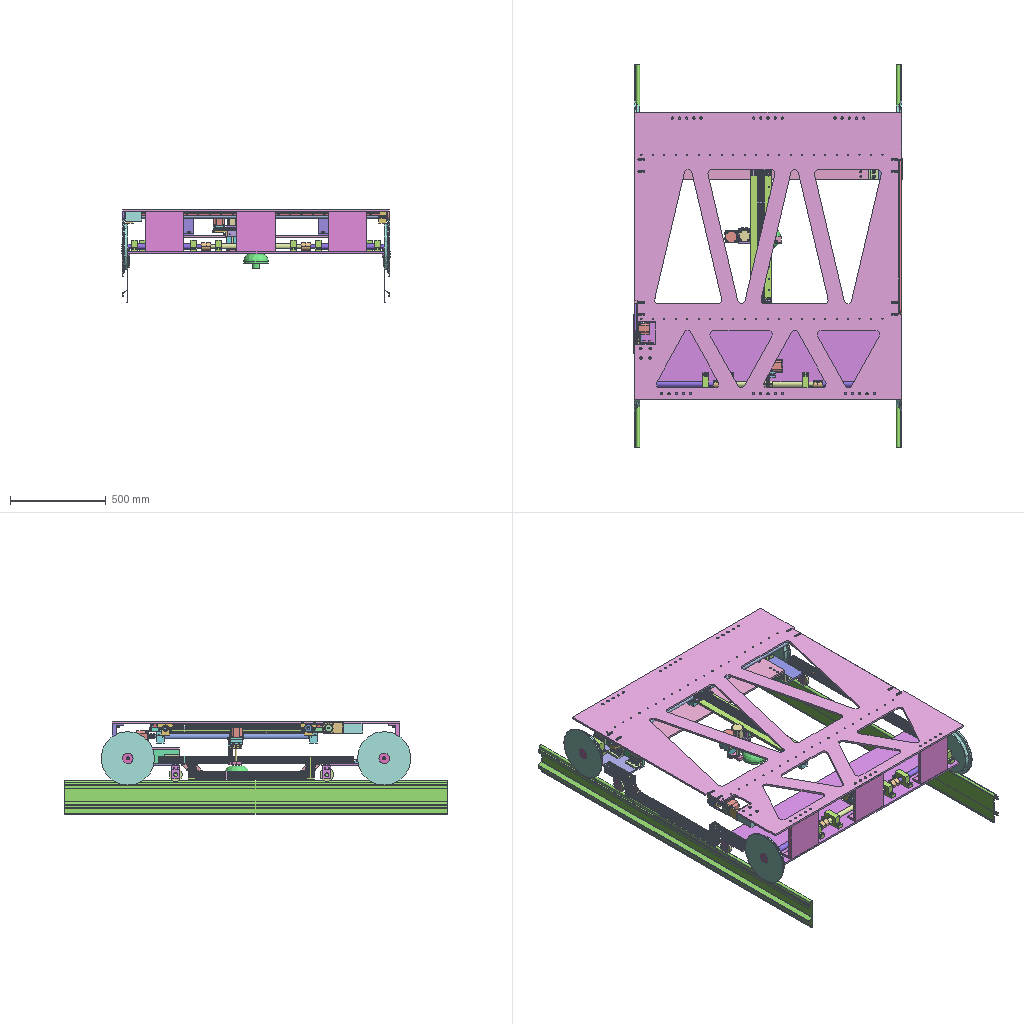Assembly | NX | 100 different items | 711 placed | box 1401 x 2000 x 485 mm
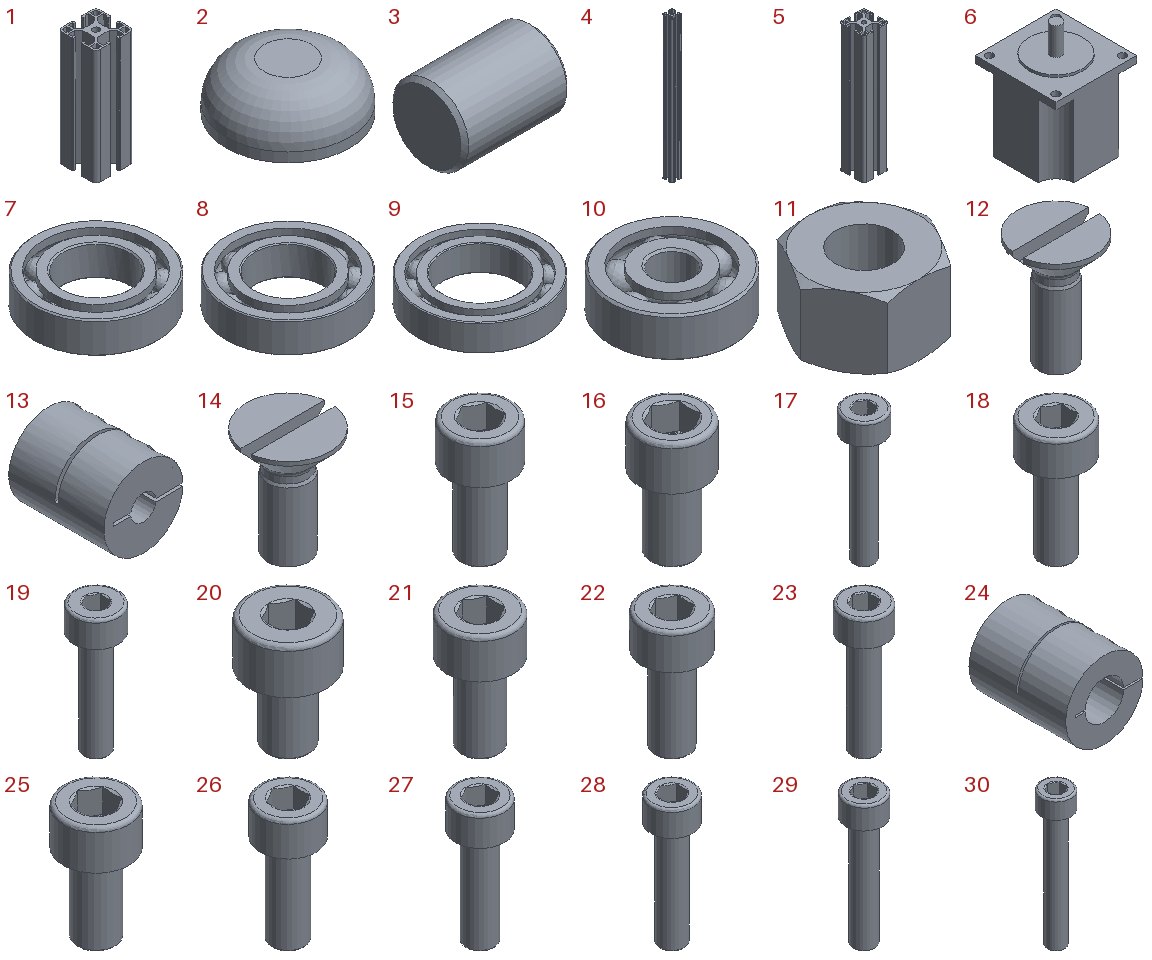Parts list (item | quantity | size | volume | features):
1 | x2 | 40 x 40 x 120 mm | 69185 mm3 | features DATUM_CSYS 2, EXTRUDE 1, SKETCH 1
2 | x1 | 130 x 130 x 80 mm | 580405 mm3 | features DATUM_CSYS 2, SKETCH 1, SWP104 1
3 | x4 | 28 x 20 x 20 mm | 8736 mm3 | features DATUM_CSYS 2, CHAMFER 1, EXTRUDE 1, SKETCH 1
4 | x1 | 40 x 40 x 580 mm | 334396 mm3 | features DATUM_CSYS 2, EXTRUDE 1, SKETCH 1
5 | x1 | 40 x 40 x 205 mm | 118192 mm3 | features DATUM_CSYS 2, EXTRUDE 1, SKETCH 1
6 | x4 | 57 x 57 x 76.9 mm | 158968 mm3 | features 57BYG350CL-SASSML-0601步进电机.SLDPRT 2
7 | x1 | 28 x 28 x 7 mm | 2050 mm3 | features SWP104 15, INSTANCE_SET 9, CHAMFER 3, SKETCH 3, DATUM_CSYS 2, FSET 2, CIRCULAR_PATTERN 1, LINE 1
8 | x6 | 37 x 37 x 9 mm | 4662 mm3 | features SWP104 16, INSTANCE_SET 10, CHAMFER 3, SKETCH 3, DATUM_CSYS 2, FSET 2, CIRCULAR_PATTERN 1, LINE 1
9 | x10 | 42 x 42 x 9 mm | 5487 mm3 | features SWP104 18, INSTANCE_SET 12, CHAMFER 3, SKETCH 3, DATUM_CSYS 2, FSET 2, CIRCULAR_PATTERN 1, LINE 1
10 | x1 | 19 x 19 x 6 mm | 1034 mm3 | features SWP104 11, INSTANCE_SET 5, CHAMFER 3, SKETCH 3, DATUM_CSYS 2, FSET 2, CIRCULAR_PATTERN 1, LINE 1
11 | x84 | 11.547 x 10 x 6.4 mm | 416.752 mm3 | features META 3, SKETCH 3, DATUM_CSYS 2, EXTRUDE 2, SWP104 2, LINE 1, SYMBOLIC_THREAD 1, THREADS 1
12 | x1 | 8.314 x 8.4 x 12 mm | 190.86 mm3 | features DATUM_CSYS 2, SKETCH 2, EXTRUDE 1, LINE 1, META 1, SWP104 1, SYMBOLIC_THREAD 1, THREADS 1
13 | x1 | 24.99 x 30 x 25 mm | 10501 mm3 | features SIMPLE HOLE 14, DATUM_CSYS 6, SYMBOLIC_THREAD 6, SKETCH 5, EXTRUDE 4, HOLE PACKAGE 3, ASSOCIATIVE_INTERSECTION 1, SWP104 1
14 | x4 | 15.673 x 15.8 x 20 mm | 1245 mm3 | features DATUM_CSYS 2, SKETCH 2, EXTRUDE 1, LINE 1, META 1, SWP104 1, SYMBOLIC_THREAD 1, THREADS 1
15 | x77 | 16 x 16 x 30 mm | 3113 mm3 | features SKETCH 3, BLEND 2, DATUM_CSYS 2, META 2, SWP104 2, CHAMFER 1, EXTRUDE 1, LINE 1, SYMBOLIC_THREAD 1, THREADS 1
16 | x55 | 18 x 18 x 32 mm | 4482 mm3 | features SKETCH 3, BLEND 2, DATUM_CSYS 2, META 2, SWP104 2, CHAMFER 1, EXTRUDE 1, LINE 1, SYMBOLIC_THREAD 1, THREADS 1
17 | x4 | 5.5 x 5.5 x 19 mm | 163.401 mm3 | features SKETCH 3, BLEND 2, DATUM_CSYS 2, META 2, SWP104 2, CHAMFER 1, EXTRUDE 1, LINE 1, SYMBOLIC_THREAD 1, THREADS 1
18 | x3 | 5.5 x 5.5 x 11 mm | 111.507 mm3 | features SKETCH 3, BLEND 2, DATUM_CSYS 2, META 2, SWP104 2, CHAMFER 1, EXTRUDE 1, LINE 1, SYMBOLIC_THREAD 1, THREADS 1
19 | x2 | 7 x 7 x 20 mm | 315.757 mm3 | features SKETCH 3, BLEND 2, DATUM_CSYS 2, META 2, SWP104 2, CHAMFER 1, EXTRUDE 1, LINE 1, SYMBOLIC_THREAD 1, THREADS 1
20 | x4 | 7 x 7 x 10 mm | 200.071 mm3 | features SKETCH 3, BLEND 2, DATUM_CSYS 2, META 2, SWP104 2, CHAMFER 1, EXTRUDE 1, LINE 1, SYMBOLIC_THREAD 1, THREADS 1
21 | x30 | 8.5 x 8.5 x 15 mm | 416.856 mm3 | features SKETCH 3, BLEND 2, DATUM_CSYS 2, META 2, SWP104 2, CHAMFER 1, EXTRUDE 1, LINE 1, SYMBOLIC_THREAD 1, THREADS 1
22 | x12 | 8.5 x 8.5 x 17 mm | 453.437 mm3 | features SKETCH 3, BLEND 2, DATUM_CSYS 2, META 2, SWP104 2, CHAMFER 1, EXTRUDE 1, LINE 1, SYMBOLIC_THREAD 1, THREADS 1
23 | x8 | 8.5 x 8.5 x 25 mm | 599.768 mm3 | features SKETCH 3, BLEND 2, DATUM_CSYS 2, META 2, SWP104 2, CHAMFER 1, EXTRUDE 1, LINE 1, SYMBOLIC_THREAD 1, THREADS 1
24 | x2 | 39.994 x 50 x 40 mm | 43416 mm3 | features SIMPLE HOLE 14, DATUM_CSYS 6, SYMBOLIC_THREAD 6, SKETCH 5, EXTRUDE 4, HOLE PACKAGE 3, ASSOCIATIVE_INTERSECTION 1, SWP104 1
25 | x26 | 10 x 10 x 18 mm | 694.735 mm3 | features SKETCH 3, BLEND 2, DATUM_CSYS 2, META 2, SWP104 2, CHAMFER 1, EXTRUDE 1, LINE 1, SYMBOLIC_THREAD 1, THREADS 1
26 | x34 | 10 x 10 x 22 mm | 800.228 mm3 | features SKETCH 3, BLEND 2, DATUM_CSYS 2, META 2, SWP104 2, CHAMFER 1, EXTRUDE 1, LINE 1, SYMBOLIC_THREAD 1, THREADS 1
27 | x101 | 10 x 10 x 26 mm | 905.721 mm3 | features SKETCH 3, BLEND 2, DATUM_CSYS 2, META 2, SWP104 2, CHAMFER 1, EXTRUDE 1, LINE 1, SYMBOLIC_THREAD 1, THREADS 1
28 | x17 | 10 x 10 x 31 mm | 1038 mm3 | features SKETCH 3, BLEND 2, DATUM_CSYS 2, META 2, SWP104 2, CHAMFER 1, EXTRUDE 1, LINE 1, SYMBOLIC_THREAD 1, THREADS 1
29 | x8 | 10 x 10 x 36 mm | 1169 mm3 | features SKETCH 3, BLEND 2, DATUM_CSYS 2, META 2, SWP104 2, CHAMFER 1, EXTRUDE 1, LINE 1, SYMBOLIC_THREAD 1, THREADS 1
30 | x24 | 10 x 10 x 46 mm | 1433 mm3 | features SKETCH 3, BLEND 2, DATUM_CSYS 2, META 2, SWP104 2, CHAMFER 1, EXTRUDE 1, LINE 1, SYMBOLIC_THREAD 1, THREADS 1
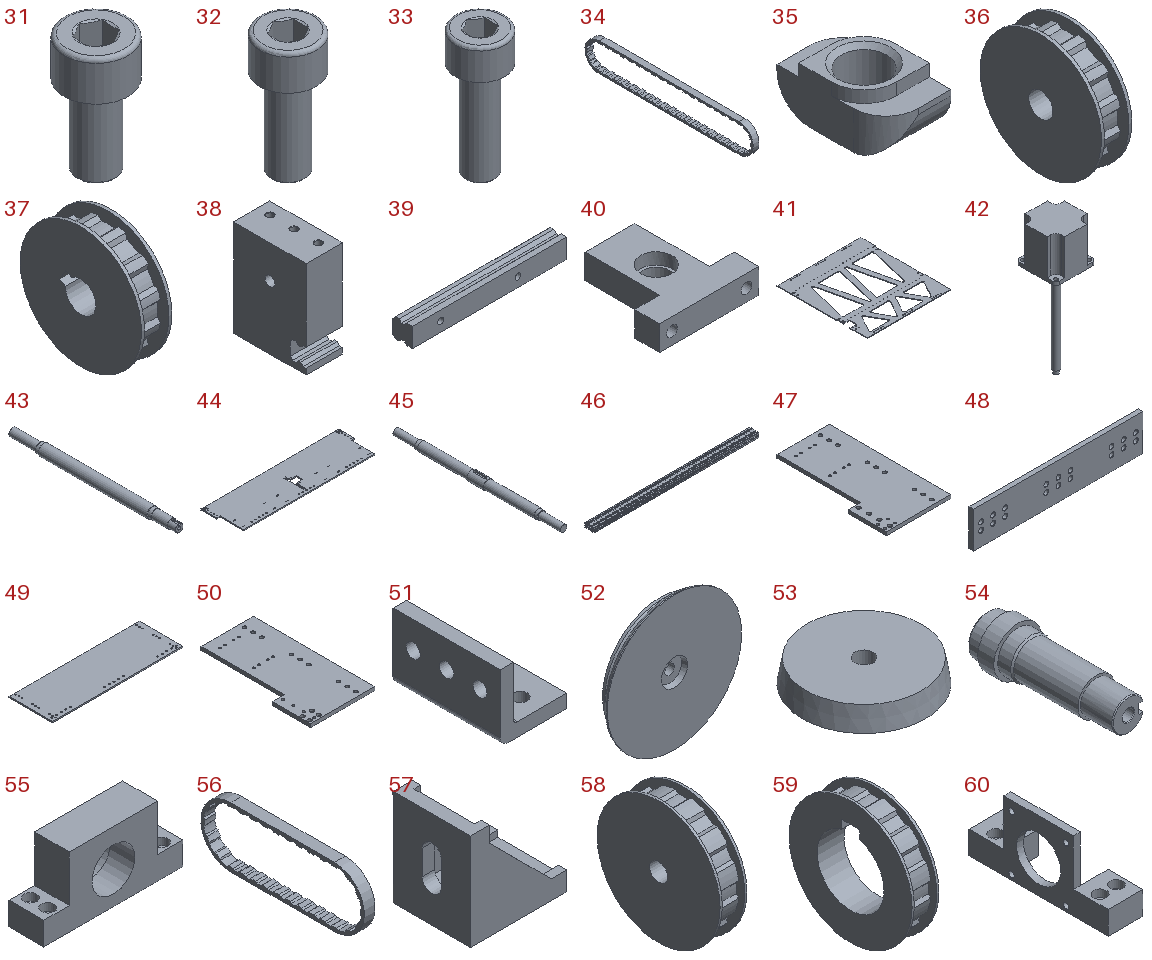31 | x3 | 13 x 13 x 24 mm | 1648 mm3 | features SKETCH 3, BLEND 2, DATUM_CSYS 2, META 2, SWP104 2, CHAMFER 1, EXTRUDE 1, LINE 1, SYMBOLIC_THREAD 1, THREADS 1
32 | x4 | 13 x 13 x 28 mm | 1837 mm3 | features SKETCH 3, BLEND 2, DATUM_CSYS 2, META 2, SWP104 2, CHAMFER 1, EXTRUDE 1, LINE 1, SYMBOLIC_THREAD 1, THREADS 1
33 | x4 | 13 x 13 x 33 mm | 2074 mm3 | features SKETCH 3, BLEND 2, DATUM_CSYS 2, META 2, SWP104 2, CHAMFER 1, EXTRUDE 1, LINE 1, SYMBOLIC_THREAD 1, THREADS 1
34 | x1 | 8 x 230.5 x 39 mm | 11364 mm3 | features CPROJ 5, DATUM_CSYS 4, EXTRUDE 3, SKETCH 3, EXTRACT_BODY 2, TRIM BODY 2, Container 1, Delete Body 1, Geometry Instance 1, Pattern Geometry 1, UNITE 1
35 | x22 | 6 x 10 x 4.6 mm | 148.977 mm3 | features DATUM_CSYS 4, SKETCH 3, EXTRUDE 2, BLEND 1, HOLE PACKAGE 1, SIMPLE HOLE 1, SYMBOLIC_THREAD 1
36 | x1 | 10 x 40 x 40 mm | 9050 mm3 | features DATUM_CSYS 3, EXTRUDE 2, SKETCH 2, Container 1, EXTRACT_BODY 1, Geometry Instance 1, UNITE 1
37 | x1 | 10 x 40 x 40 mm | 8689 mm3 | features DATUM_CSYS 4, EXTRUDE 3, SKETCH 3, Container 1, EXTRACT_BODY 1, Geometry Instance 1, UNITE 1
38 | x1 | 30 x 60 x 80 mm | 135184 mm3 | features CBORE_HOLE 8, DATUM_CSYS 6, SYMBOLIC_THREAD 6, SIMPLE HOLE 5, SKETCH 5, HOLE PACKAGE 3, EXTRUDE 2, SUBTRACT 1
39 | x1 | 120 x 15 x 15 mm | 23818 mm3 | features CBORE_HOLE 8, DATUM_CSYS 3, EXTRUDE 2, SKETCH 2, HOLE PACKAGE 1
40 | x1 | 60 x 60 x 15 mm | 28357 mm3 | features DATUM_CSYS 4, SKETCH 3, CBORE_HOLE 2, EXTRUDE 2, HOLE PACKAGE 1
41 | x1 | 1395 x 1500 x 10 mm | 12886681 mm3 | features SIMPLE HOLE 74, SYMBOLIC_THREAD 74, DATUM_CSYS 61, SKETCH 60, EXTRACT_FACE 55, HOLE PACKAGE 55, Instance Feature 49, CBORE_HOLE 28, EXTRACT_DATUM_PLANE 7, EXTRUDE 6, Pattern Feature 6
42 | x1 | 56.4 x 56.4 x 188.6 mm | 156156 mm3 | features DATUM_CSYS 7, EXTRUDE 6, SKETCH 6, BLEND 1, DISTANCE MEASUREMENT 1, SYMBOLIC_THREAD 1
43 | x2 | 28 x 428 x 28 mm | 224992 mm3 | features DATUM_CSYS 3, CHAMFER 2, EXTRUDE 2, SKETCH 2, FACE_BLEND 1, HOLE PACKAGE 1, SIMPLE HOLE 1, SWP104 1, SYMBOLIC_THREAD 1
44 | x1 | 1400 x 400 x 10 mm | 5316360 mm3 | features SIMPLE HOLE 43, SYMBOLIC_THREAD 43, CBORE_HOLE 18, DATUM_CSYS 18, EXTRACT_FACE 17, SKETCH 17, HOLE PACKAGE 15, Instance Feature 6, EXTRUDE 2, Mirror Feature 2, Pattern Feature 1
45 | x1 | 30 x 520 x 30 mm | 265320 mm3 | features DATUM_CSYS 3, SKETCH 2, EXTRUDE 1, SWP104 1
46 | x1 | 700 x 40 x 20 mm | 206899 mm3 | features DATUM_CSYS 2, EXTRUDE 1, SKETCH 1
47 | x1 | 185.5 x 350 x 10 mm | 550667 mm3 | features SIMPLE HOLE 25, SYMBOLIC_THREAD 17, DATUM_CSYS 10, HOLE PACKAGE 9, SKETCH 9, EXTRACT_FACE 6, CBORE_HOLE 4, Instance Feature 4, Pattern Feature 2, EXTRUDE 1
48 | x2 | 350 x 10 x 75 mm | 250917 mm3 | features SIMPLE HOLE 18, SYMBOLIC_THREAD 18, DATUM_CSYS 4, SKETCH 3, EXTRACT_DATUM_AXIS 2, EXTRACT_FACE 2, HOLE PACKAGE 2, EXTRUDE 1, Instance Feature 1, Mirror Feature 1
49 | x1 | 1050 x 350 x 10 mm | 3649259 mm3 | features SIMPLE HOLE 33, SYMBOLIC_THREAD 33, DATUM_CSYS 5, SKETCH 4, HOLE PACKAGE 3, EXTRACT_FACE 2, EXTRUDE 1, Instance Feature 1, Mirror Feature 1
50 | x1 | 184.5 x 350 x 10 mm | 549567 mm3 | features SIMPLE HOLE 25, SYMBOLIC_THREAD 17, DATUM_CSYS 10, HOLE PACKAGE 9, SKETCH 9, EXTRACT_FACE 6, CBORE_HOLE 4, Instance Feature 4, Pattern Feature 2, EXTRUDE 1
51 | x12 | 50 x 80 x 50 mm | 66341 mm3 | features SIMPLE HOLE 6, DATUM_CSYS 4, SKETCH 3, BLEND 2, EXTRACT_DATUM_AXIS 2, EXTRACT_FACE 2, HOLE PACKAGE 2, EXTRUDE 1, Instance Feature 1, Mirror Feature 1
52 | x4 | 280 x 30 x 280 mm | 1461901 mm3 | features DATUM_CSYS 5, SKETCH 4, EXTRUDE 3, CPROJ 1, Delete Body 1, HOLE PACKAGE 1, SIMPLE HOLE 1, SWP104 1
53 | x4 | 55 x 55 x 10 mm | 21401 mm3 | features DATUM_CSYS 3, SKETCH 2, ASSOCIATIVE_INTERSECTION 1, EXTRUDE 1, SWP104 1
54 | x2 | 30 x 88 x 30 mm | 37691 mm3 | features DATUM_CSYS 3, EXTRUDE 3, CHAMFER 2, SKETCH 2, FACE_BLEND 1, HOLE PACKAGE 1, SIMPLE HOLE 1, SWP104 1, SYMBOLIC_THREAD 1
55 | x10 | 120 x 30 x 60 mm | 123889 mm3 | features CBORE_HOLE 4, DATUM_CSYS 4, SKETCH 3, EXTRUDE 2, HOLE PACKAGE 1
56 | x1 | 10 x 150 x 55 mm | 11245 mm3 | features CPROJ 6, DATUM_CSYS 4, EXTRUDE 3, SKETCH 3, EXTRACT_BODY 2, TRIM BODY 2, Container 1, Delete Body 1, Geometry Instance 1, Pattern Geometry 1, UNITE 1
57 | x4 | 35 x 28 x 35 mm | 9798 mm3 | features DATUM_CSYS 6, SKETCH 5, EXTRACT_DATUM_AXIS 4, EXTRACT_FACE 4, EXTRACT_STRING 4, EXTRUDE 4, Instance Feature 2, Mirror Feature 1, Pattern Feature 1, Variational Failed Derived Feature With Body 1
58 | x1 | 12 x 55 x 55 mm | 22955 mm3 | features DATUM_CSYS 3, EXTRUDE 2, SKETCH 2, Container 1, EXTRACT_BODY 1, Geometry Instance 1, UNITE 1
59 | x1 | 12 x 55 x 55 mm | 14742 mm3 | features DATUM_CSYS 4, EXTRUDE 3, SKETCH 3, Container 1, EXTRACT_BODY 1, Geometry Instance 1, UNITE 1
60 | x1 | 30 x 120 x 60 mm | 46111 mm3 | features DATUM_CSYS 5, CBORE_HOLE 4, SIMPLE HOLE 4, SKETCH 4, SYMBOLIC_THREAD 4, EXTRUDE 3, HOLE PACKAGE 2
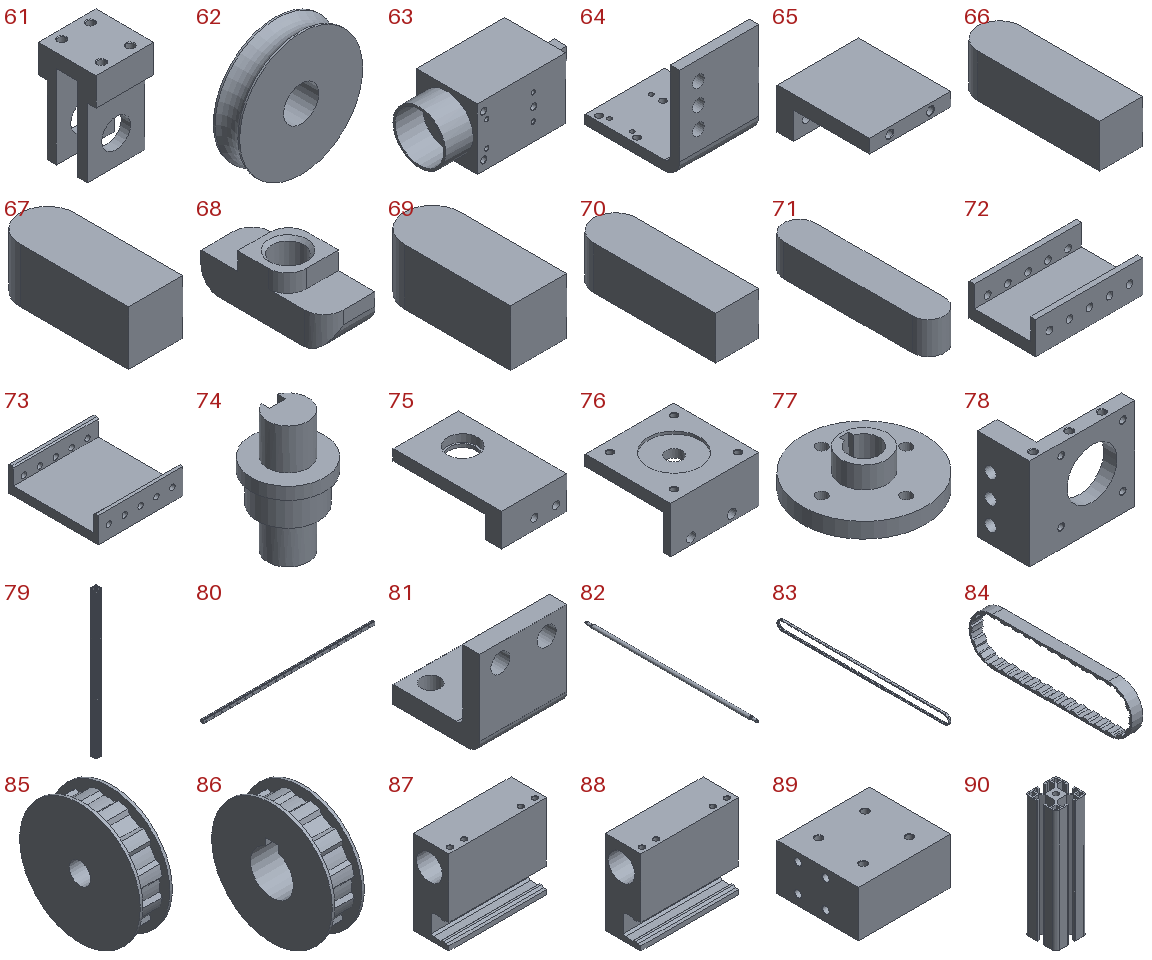61 | x4 | 40 x 40 x 67.571 mm | 44865 mm3 | features SIMPLE HOLE 5, DATUM_CSYS 4, SYMBOLIC_THREAD 4, SKETCH 3, EXTRUDE 2, HOLE PACKAGE 2
62 | x4 | 70 x 15 x 70 mm | 48198 mm3 | features DATUM_CSYS 3, SKETCH 2, Delete Body 1, EXTRUDE 1, SWP104 1
63 | x1 | 61 x 29 x 29 mm | 36377 mm3 | features SIMPLE HOLE 7, SYMBOLIC_THREAD 7, DATUM_CSYS 6, SKETCH 5, EXTRUDE 4, HOLE PACKAGE 2
64 | x1 | 42 x 50 x 50 mm | 18797 mm3 | features SIMPLE HOLE 10, DATUM_CSYS 5, SKETCH 4, HOLE PACKAGE 3, EXTRUDE 1
65 | x1 | 60 x 68 x 30 mm | 53216 mm3 | features SIMPLE HOLE 5, DATUM_CSYS 4, SKETCH 3, HOLE PACKAGE 2, SYMBOLIC_THREAD 2, EXTRUDE 1
66 | x1 | 3 x 10 x 3 mm | 87.103 mm3 | features DATUM_CSYS 2, EXTRUDE 1, SKETCH 1
67 | x1 | 4 x 10 x 4 mm | 153.133 mm3 | features DATUM_CSYS 2, EXTRUDE 1, FACE_BLEND 1, SKETCH 1
68 | x26 | 8 x 19.3 x 7.8 mm | 733.523 mm3 | features DATUM_CSYS 4, SKETCH 3, EXTRUDE 2, BLEND 1, HOLE PACKAGE 1, SIMPLE HOLE 1, SYMBOLIC_THREAD 1
69 | x3 | 5 x 12 x 5 mm | 286.587 mm3 | features DATUM_CSYS 2, EXTRUDE 1, FACE_BLEND 1, SKETCH 1
70 | x4 | 6 x 20 x 6 mm | 696.823 mm3 | features DATUM_CSYS 2, EXTRUDE 1, FACE_BLEND 1, SKETCH 1
71 | x1 | 8 x 40 x 8 mm | 2450 mm3 | features DATUM_CSYS 2, EXTRUDE 1, SKETCH 1
72 | x3 | 200 x 125 x 60 mm | 647728 mm3 | features EXTRACT_BODY 5, SIMPLE HOLE 5, DATUM_CSYS 3, EXTRUDE 2, SKETCH 2, CHAMFER 1, Container 1, Geometry Instance 1, HOLE PACKAGE 1, SUBTRACT 1
73 | x3 | 200 x 210 x 60 mm | 985928 mm3 | features SIMPLE HOLE 15, DATUM_CSYS 7, SKETCH 6, EXTRACT_BODY 5, EXTRACT_DATUM_AXIS 5, EXTRACT_FACE 5, HOLE PACKAGE 5, Instance Feature 4, CHAMFER 2, Delete Body 2, EXTRUDE 2, Container 1, Geometry Instance 1, Pattern Feature 1, SUBTRACT 1
74 | x1 | 18 x 18 x 30 mm | 3301 mm3 | features DATUM_CSYS 4, SKETCH 3, EXTRUDE 2, FACE_BLEND 1, HOLE PACKAGE 1, SIMPLE HOLE 1, SUBTRACT 1, SWP104 1, SYMBOLIC_THREAD 1
75 | x1 | 60 x 100 x 30 mm | 70418 mm3 | features DATUM_CSYS 4, HOLE PACKAGE 3, SKETCH 3, CBORE_HOLE 2, SIMPLE HOLE 2, EXTRUDE 1
76 | x1 | 65 x 63 x 34 mm | 37407 mm3 | features SIMPLE HOLE 7, DATUM_CSYS 5, EXTRUDE 4, SKETCH 4, SYMBOLIC_THREAD 4, HOLE PACKAGE 3
77 | x1 | 40 x 40 x 12 mm | 5639 mm3 | features SIMPLE HOLE 5, DATUM_CSYS 4, SYMBOLIC_THREAD 4, SKETCH 3, CPROJ 2, HOLE PACKAGE 2, EXTRUDE 1, SWP104 1
78 | x1 | 80 x 40 x 70 mm | 69498 mm3 | features SIMPLE HOLE 8, SYMBOLIC_THREAD 7, DATUM_CSYS 6, SKETCH 5, HOLE PACKAGE 4, CBORE_HOLE 3, EXTRUDE 3
79 | x1 | 40 x 40 x 1020 mm | 588076 mm3 | features DATUM_CSYS 2, EXTRUDE 1, SKETCH 1
80 | x2 | 1328 x 22 x 23 mm | 615585 mm3 | features CBORE_HOLE 22, DATUM_CSYS 3, SKETCH 2, EXTRUDE 1, HOLE PACKAGE 1
81 | x4 | 30 x 30 x 30 mm | 8846 mm3 | features DATUM_CSYS 3, EXTRACT_BODY 2, SIMPLE HOLE 2, SKETCH 2, BLEND 1, Container 1, EXTRUDE 1, Geometry Instance 1, HOLE PACKAGE 1, SUBTRACT 1
82 | x2 | 28 x 1395 x 28 mm | 817167 mm3 | features CHAMFER 4, DATUM_CSYS 3, SKETCH 2, Container 1, EXTRACT_BODY 1, EXTRUDE 1, FACE_BLEND 1, Geometry Instance 1, SUBTRACT 1, SWP104 1, SYMBOLIC_THREAD 1
83 | x1 | 10 x 791 x 43 mm | 37818 mm3 | features CPROJ 5, DATUM_CSYS 4, EXTRUDE 3, SKETCH 3, EXTRACT_BODY 2, TRIM BODY 2, Container 1, Delete Body 1, Geometry Instance 1, Pattern Geometry 1, UNITE 1
84 | x1 | 10 x 149 x 43 mm | 7788 mm3 | features CPROJ 5, DATUM_CSYS 4, EXTRUDE 3, SKETCH 3, EXTRACT_BODY 2, TRIM BODY 2, Container 1, Delete Body 1, Geometry Instance 1, Pattern Geometry 1, UNITE 1
85 | x1 | 12 x 45 x 45 mm | 14319 mm3 | features DATUM_CSYS 3, EXTRUDE 2, SKETCH 2, Container 1, EXTRACT_BODY 1, Geometry Instance 1, UNITE 1
86 | x3 | 12 x 45 x 45 mm | 12364 mm3 | features DATUM_CSYS 4, EXTRUDE 3, SKETCH 3, Container 1, EXTRACT_BODY 1, Geometry Instance 1, UNITE 1
87 | x1 | 110 x 40 x 95 mm | 307635 mm3 | features SIMPLE HOLE 10, SYMBOLIC_THREAD 9, DATUM_CSYS 5, HOLE PACKAGE 4, SKETCH 4, EXTRUDE 2, SUBTRACT 1
88 | x1 | 110 x 40 x 95 mm | 303623 mm3 | features SIMPLE HOLE 14, SYMBOLIC_THREAD 13, DATUM_CSYS 6, HOLE PACKAGE 5, SKETCH 5, EXTRUDE 2, SUBTRACT 1
89 | x1 | 100 x 88 x 50 mm | 433073 mm3 | features SIMPLE HOLE 8, SYMBOLIC_THREAD 8, DATUM_CSYS 4, SKETCH 3, HOLE PACKAGE 2, EXTRUDE 1
90 | x1 | 40 x 40 x 155 mm | 89365 mm3 | features DATUM_CSYS 2, EXTRUDE 1, SKETCH 1
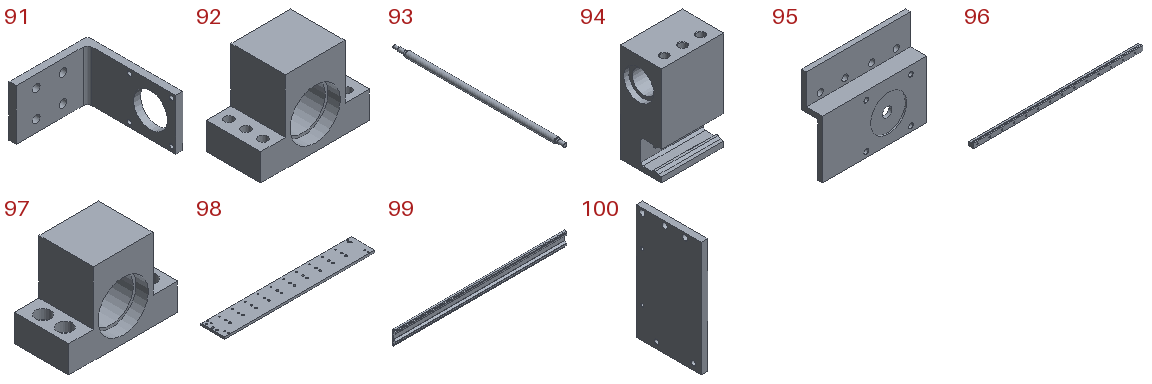91 | x1 | 88 x 107 x 57 mm | 73823 mm3 | features SIMPLE HOLE 9, DATUM_CSYS 6, SKETCH 5, SYMBOLIC_THREAD 4, EXTRUDE 3, HOLE PACKAGE 3, BLEND 1
92 | x4 | 80 x 40 x 60 mm | 94227 mm3 | features SIMPLE HOLE 6, DATUM_CSYS 5, SKETCH 4, EXTRUDE 2, HOLE PACKAGE 2, CBORE_HOLE 1
93 | x1 | 28 x 865 x 28 mm | 492482 mm3 | features CHAMFER 2, DATUM_CSYS 2, SKETCH 1, SWP104 1, SYMBOLIC_THREAD 1, TRIM BODY 1
94 | x1 | 60 x 40 x 95 mm | 172371 mm3 | features SIMPLE HOLE 8, SYMBOLIC_THREAD 7, DATUM_CSYS 5, HOLE PACKAGE 4, SKETCH 4, EXTRUDE 2, SUBTRACT 1
95 | x1 | 110 x 22 x 93 mm | 57423 mm3 | features SIMPLE HOLE 10, DATUM_CSYS 5, SKETCH 4, SYMBOLIC_THREAD 4, HOLE PACKAGE 3, EXTRUDE 2
96 | x1 | 840 x 22 x 23 mm | 392391 mm3 | features CBORE_HOLE 14, DATUM_CSYS 3, SKETCH 2, EXTRUDE 1, HOLE PACKAGE 1
97 | x2 | 80 x 40 x 60 mm | 93822 mm3 | features CBORE_HOLE 5, DATUM_CSYS 5, SKETCH 4, EXTRUDE 2, HOLE PACKAGE 2
98 | x1 | 700 x 110 x 10 mm | 755648 mm3 | features CBORE_HOLE 22, SIMPLE HOLE 20, SYMBOLIC_THREAD 20, DATUM_CSYS 15, SKETCH 14, HOLE PACKAGE 13, EXTRACT_DATUM_PLANE 11, EXTRACT_FACE 11, Instance Feature 10, EXTRUDE 1, Pattern Feature 1
99 | x2 | 2000 x 29.98 x 174.62 mm | 1173848 mm3 | features DATUM_CSYS 2, EXTRUDE 1, SKETCH 1
100 | x1 | 8 x 80 x 141 mm | 88943 mm3 | features SIMPLE HOLE 7, DATUM_CSYS 5, SKETCH 4, SYMBOLIC_THREAD 4, HOLE PACKAGE 3, EXTRUDE 1
Mates (type | each side: item.copy, entity, surface, feature), first 324 of 427 lines:
Center12 | 41.1 face plane Extrude(1) | 41.1 | assembly plane
Center12 | 41.1 face plane Extrude(1) | 41.1 face plane Extrude(1) | assembly plane
Touch | 41.1 face plane Extrude(1) | assembly plane
Touch | 92.1 face plane Extrude(1) | 41.1 face plane Extrude(1) | 3 times
Parallel | 92.1 face plane Extrude(1) | 41.1 face plane Extrude(1)
Distance | 92.1 face plane Extrude(1) | 41.1
Touch | 82.1 face cylinder Revolve(1) | 92.1 face cylinder Ø33 Counterbored Hole(2)
Touch | 8.1 face plane Revolve(6) | 92.1 face plane Ø33 Counterbored Hole(2) | 2 times
Touch | 8.1 face surfaceofrevolution Revolve(8) | 92.1 face cylinder Ø33 Counterbored Hole(2)
Touch | 82.1 face plane Revolve(1) | 8.1 face plane Revolve(6) | 2 times
Touch | 92.1 face plane Extrude(1) | 92.1 face plane Extrude(1) | 4 times
Touch | 8.1 face plane Revolve(6) | 82.1 face plane Revolve(1) | 2 times
Touch | 8.1 face cylinder Revolve(6) | 82.1 face cylinder Revolve(1) | 2 times
Touch | 92.1 face plane Ø33 Counterbored Hole(2) | 8.1 face plane Revolve(6) | 2 times
Touch | 80.1 face plane Extrude(1) | 41.1 face plane Extrude(1)
Distance | 80.1 face plane Extrude(1) | 92.1 face plane Extrude(1)
Touch | 81.1 face plane Extrude(1) | 98.1 face plane Extrude(1) | 8 times
Touch | 8.1 face plane Revolve(6) | 97.1 face plane Ø33 Counterbored Hole(2)
Touch | 8.1 face cylinder Revolve(5) | 97.1 face cylinder Ø33 Counterbored Hole(2)
Touch | 93.1 face cylinder Revolve(1) | 97.1 face cylinder Ø33 Counterbored Hole(2) | 2 times
Touch | 93.1 face plane Revolve(1) | 8.1 face plane Revolve(6)
Touch | 96.1 face plane Extrude(1) | 98.1 face plane Extrude(1)
Touch | 96.1 face plane Extrude(1) | 97.1 face plane Extrude(1)
Touch | 94.1 face cylinder Extrude(2) | 93.1 face cylinder Revolve(1)
Touch | 96.1 face plane Extrude(1) | 94.1 face plane Extrude(1)
Touch | 78.1 face plane Extrude(1) | 94.1 face plane Extrude(2) | 3 times
Parallel | 78.1 face plane Extrude(1) | 94.1 face plane Extrude(2)
Touch | 42.1 face plane Extrude(1) | 78.1 face plane Extrude(3)
Touch | 42.1 face cylinder Extrude(5) | 78.1 face cylinder Ø38.1 Hole(2)
Parallel | 42.1 face plane Extrude(1) | 78.1 face plane Extrude(1)
Touch | 100.1 face plane Extrude(1) | 78.1 face plane Extrude(3)
Touch | 100.1 face plane Extrude(1) | 78.1 face plane Extrude(1)
Touch | 40.1 face plane Extrude(1) | 100.1 face plane Extrude(1) | 2 times
Touch | 10.1 face cylinder Revolve(6) | 42.1 face cylinder Extrude(7)
Touch | 10.1 face plane Revolve(6) | 42.1 face plane Extrude(5)
Touch | 39.1 face plane Extrude(1) | 100.1 face plane Extrude(1) | 2 times
Touch | 100.1 face plane Extrude(1) | 78.1 face plane Extrude(5)
Touch | 38.1 face plane Extrude(1) | 39.1 face plane Extrude(1)
Parallel | 38.1 face plane Extrude(3) | 100.1 face plane Extrude(1)
Distance | 78.1 face plane Extrude(1) | 38.1 face plane Extrude(3)
Touch | 65.1 face plane Extrude(1) | 38.1 face plane Extrude(3) | 3 times
Touch | 76.1 | 65.1 face plane Extrude(1) | 2 times
Touch | 76.1 edge | 65.1 face plane Extrude(1)
Touch | 6.1 face plane 57BYG350CL-SASSML-0601步进电机.SLDPRT(1) | 76.1 face plane Extrude(1)
Touch | 76.1 face cylinder Ø12 Hole(3) | 6.1 face cylinder 57BYG350CL-SASSML-0601步进电机.SLDPRT(1)
Parallel | 6.1 face plane 57BYG350CL-SASSML-0601步进电机.SLDPRT(1) | 76.1
Touch | 75.1 face plane Extrude(1) | 38.1 face plane Extrude(3) | 3 times
Touch | 74.1 face plane Revolve(1) | 75.1 face plane Extrude(1)
Touch | 74.1 face cylinder Revolve(1) | 75.1 face cylinder Ø28 Hole(2)
Touch | 7.1 face cylinder Revolve(5) | 74.1 face cylinder Revolve(1)
Touch | 7.1 face plane Revolve(6) | 74.1 face plane Revolve(1)
Touch | 77.1 face cylinder Revolve(1) | 74.1 face cylinder Revolve(1)
Touch | 38.1 face cylinder Extrude(3) | 42.1 face cylinder Extrude(5)
Touch | 54.1 face cylinder Revolve(1) | 52.1 face cone Extrude(4)
Touch | 54.1 face plane Revolve(1) | 52.1 face plane Extrude(4)
Touch | 52.1 face plane Extrude(6) | 54.1 face plane Extrude(2) | 2 times
Touch | 52.1 face surfaceofrevolution Revolve(2) | 99.1 face cylinder Extrude(1) | 3 times
Touch | 49.1 face plane Extrude(1) | 48.1 face plane Extrude(1) | 2 times
Touch | 48.1 face plane Extrude(1) | 49.1 face plane Extrude(1) | 4 times
Touch | 47.1 face plane Extrude(1) | 48.1 face plane Extrude(1) | 3 times
Touch | 54.1 face cylinder Revolve(1) | 52.1 face cylinder Ø20 Hole(5)
Touch | 9.1 face cylinder Revolve(5) | 54.1 face cylinder Revolve(1)
Touch | 52.1 face plane Extrude(4) | 54.1 face plane Revolve(1)
Distance | 99.1 face plane Extrude(1) | 47.1 face plane Extrude(1)
Parallel | 49.1 face plane Extrude(1) | assembly plane | 2 times
Distance | assembly plane | 49.1 face plane Extrude(1)
Touch | 54.1 | 9.1 face plane Revolve(6)
Center12 | 52.1 face plane Revolve(2) | 52.1 face plane Revolve(2) | assembly plane
Parallel | 52.1 face plane Extrude(6) | 48.1 face plane Extrude(1) | 2 times
Touch | 52.1 face plane Revolve(2) | 52.1 face plane Revolve(2) | 3 times
Parallel | 52.1 face plane Extrude(6) | assembly plane
Touch | 43.1 face plane Revolve(1) | 52.1 face plane Extrude(4)
Touch | 43.1 face cylinder Revolve(1) | 52.1 face cylinder Ø20 Hole(5)
Touch | 43.1 face plane Extrude(2) | 52.1 face plane Extrude(6)
Parallel | 44.1 face plane Extrude(1) | assembly plane
Distance | 44.1 face plane Extrude(1) | assembly plane | 2 times
Touch | 55.1 face cylinder Extrude(2) | 43.1 face cylinder Revolve(1) | 4 times
Touch | 9.1 face plane Revolve(6) | 43.1 face plane Revolve(1) | 2 times
Touch | 9.1 face cylinder Revolve(5) | 43.1 face cylinder Revolve(1) | 2 times
Touch | 9.1 face plane Revolve(6) | 43.1 | 2 times
Touch | 9.1 face surfaceofrevolution Revolve(7) | 43.1 face cylinder Revolve(1)
Touch | 55.1 face plane Extrude(2) | 9.1 face plane Revolve(6) | 2 times
Parallel | 55.1 face plane Extrude(1) | assembly plane
Distance | 44.1 face plane Extrude(1) | 55.1 face plane Extrude(1)
Touch | 24.1 face cylinder Revolve(1) | 43.1 face cylinder Revolve(1) | 2 times
Parallel | 24.1 face plane Extrude(6) | assembly plane
Touch | 45.1 face cylinder Revolve(1) | 24.1 face cylinder Revolve(1)
Touch | 37.1 face cylinder Extrude(1) | 74.1 face cylinder Revolve(1)
Touch | 37.1 face plane Extrude(2) | 74.1 face plane Revolve(1)
Touch | 36.1 face cylinder Extrude(1) | 6.1 face cylinder 57BYG350CL-SASSML-0601步进电机.SLDPRT(1)
Touch | 36.1 face plane Extrude(2) | 6.1 face plane 57BYG350CL-SASSML-0601步进电机.SLDPRT(1)
Touch | 34.1 face plane Extrude(8) | 37.1 face plane Extrude(2)
Touch | 34.1 face cylinder Extrude(8) | 37.1 face cylinder Mirror Geometry(3)
Touch | 34.1 face cylinder Extrude(8) | 36.1 face cylinder Extrude(1)
Touch | 98.1 face plane Extrude(1) | 81.1 face plane Extrude(1) | 2 times
Touch | 81.1 face plane Extrude(1) | 98.1 edge
Touch | 24.1 face cylinder Revolve(1) | 45.1 face cylinder Revolve(1)
Touch | 24.1 face plane Extrude(2) | 45.1 face plane Revolve(1)
Parallel | 24.1 face plane Extrude(6) | 44.1 face plane Extrude(1)
Touch | 43.1 face plane Revolve(1) | 24.1 face plane Extrude(2) | 2 times
Touch | 52.1 face plane Extrude(6) | 43.1 face plane Extrude(2)
Touch | 52.1 face cylinder Ø20 Hole(5) | 43.1 face cylinder Revolve(1)
Touch | 52.1 face plane Extrude(4) | 43.1 face plane Revolve(1)
Touch | 9.1 face cylinder Revolve(6) | 43.1 face cylinder Revolve(1)
Touch | 55.1 face plane Extrude(1) | 44.1 face plane Extrude(1) | 5 times
Distance | 55.1 face plane Extrude(1) | 44.1 face plane Extrude(1) | 2 times
Touch | 9.1 face plane Revolve(5) | 55.1 face plane Extrude(2)
Touch | 9.1 face plane Revolve(6) | 55.1 face plane Extrude(2)
Touch | 87.1 face plane Extrude(2) | 81.1 face plane Extrude(1)
Touch | 87.1 face plane Extrude(2) | 98.1 face plane Extrude(1) | 2 times
Touch | 82.1 face cylinder Revolve(1) | 87.1 face cylinder Extrude(2)
Touch | 80.1 face plane Extrude(1) | 87.1 face plane Extrude(1) | 2 times
Touch | 80.1 face plane Extrude(1) | 92.1 face plane Extrude(1) | 2 times
Touch | 8.1 face cone Chamfer(34) | 82.1 face cylinder Revolve(1)
Touch | 8.1 face plane Revolve(6) | 93.1 face plane Revolve(1)
Touch | 97.1 face plane Ø33 Counterbored Hole(2) | 8.1 face plane Revolve(6)
Touch | 8.1 face cylinder Revolve(6) | 97.1 face cylinder Ø33 Counterbored Hole(2)
Touch | 97.1 face plane Extrude(1) | 87.1 face plane Extrude(2) | 2 times
Touch | 62.1 face surfaceofrevolution Revolve(3) | 61.1 face cylinder Ø20 Hole(2) | 2 times
Touch | 62.1 face plane Revolve(3) | 61.1 face plane Extrude(1) | 4 times
Touch | 62.1 face surfaceofrevolution Revolve(3) | 99.1 face cylinder Extrude(1)
Touch | 61.1 face plane Extrude(1) | 44.1 face plane Extrude(1) | 3 times
Touch | 61.1 face plane Extrude(3) | 44.1 face plane Extrude(1) | 2 times
Touch | 62.1 face cylinder Revolve(3) | 61.1 face cylinder Ø20 Hole(2) | 2 times
Touch | 61.1 face plane Extrude(1) | 47.1 face plane Extrude(1) | 2 times
Touch | 61.1 face plane Extrude(3) | 47.1 face plane Extrude(1)
Touch | 92.1 face plane Extrude(1) | 80.1 face plane Extrude(1)
Touch | 92.1 face cylinder Ø33 Counterbored Hole(2) | 82.1 face cylinder Revolve(1)
Touch | 86.1 face cylinder Extrude(2) | 82.1 face cylinder Revolve(1)
Touch | 86.1 face plane Extrude(2) | 82.1 face plane Revolve(1)
Touch | 86.1 face plane Mirror Geometry(3) | 82.1 face plane Revolve(1)
Touch | 86.1 face cylinder Extrude(1) | 82.1 face cylinder Revolve(1) | 2 times
Touch | 86.1 face plane Extrude(2) | 82.1
Touch | 83.1 face cylinder Extrude(8) | 86.1 face cylinder Extrude(2)
Touch | 83.1 face plane Extrude(8) | 86.1 face plane Extrude(2)
Touch | 86.1 face cylinder Extrude(1) | 83.1 face cylinder Extrude(8)
Touch | 86.1 face plane Extrude(2) | 41.1 face plane Extrude(1)
Touch | 6.1 face plane 57BYG350CL-SASSML-0601步进电机.SLDPRT(1) | 86.1 face plane Mirror Geometry(3)
Touch | 85.1 face plane Mirror Geometry(3) | 6.1 face plane 57BYG350CL-SASSML-0601步进电机.SLDPRT(1)
Touch | 85.1 face cylinder Extrude(1) | 6.1 face cylinder 57BYG350CL-SASSML-0601步进电机.SLDPRT(1)
Touch | 84.1 face cylinder Extrude(8) | 86.1 face cylinder Extrude(2)
Touch | 84.1 face plane Extrude(8) | 86.1 face plane Mirror Geometry(3)
Parallel | 84.1 face plane Extrude(8) | assembly plane
Touch | 84.1 face cylinder Extrude(8) | 85.1 face cylinder Mirror Geometry(3)
Touch | 92.1 face cylinder Ø33 Counterbored Hole(2) | 8.1 face cylinder Revolve(5)
Touch | 92.1 face plane Extrude(1) | 8.1 face plane Revolve(5)
Touch | 91.1 face plane Extrude(1) | 6.1 face plane 57BYG350CL-SASSML-0601步进电机.SLDPRT(1) | 3 times
Parallel | 6.1 face plane 57BYG350CL-SASSML-0601步进电机.SLDPRT(1) | 41.1 face plane Extrude(1)
Parallel | 91.1 face plane Extrude(1) | 41.1 face plane Extrude(1)
Touch | 89.1 face plane Extrude(1) | 91.1 face plane Extrude(2)
Touch | 91.1 face plane Extrude(1) | 89.1 face plane Extrude(1)
Touch | 89.1 face plane Extrude(1) | 41.1 face plane Extrude(1)
Touch | 53.1 face plane Extrude(1) | 52.1 face plane Extrude(4) | 4 times
Touch | 53.1 face cone Extrude(1) | 52.1 face cone Extrude(4) | 4 times
Parallel | 99.1 face plane Extrude(1) | assembly plane | 2 times
Touch | 99.1 face plane Extrude(1) | 99.1 face plane Extrude(1)
Touch | 39.1 face plane Extrude(1) | 40.1 face plane Extrude(1)
Touch | 3.1 face cylinder Extrude(1) | 61.1 face cylinder Ø20 Hole(2) | 2 times
Touch | 3.1 face plane Extrude(1) | 61.1 face plane Extrude(1) | 4 times
Touch | 3.1 face cylinder Extrude(1) | 62.1 face cylinder Revolve(3) | 2 times
Center22 | 46.1 face plane Extrude(1) | 46.1 face plane Extrude(1) | 98.1 face plane Extrude(1) | 98.1 face plane Extrude(1)
Touch | 98.1 face plane Extrude(1) | 46.1 face plane Extrude(1)
Touch | 79.1 face plane Extrude(1) | 44.1 face plane Extrude(1) | 3 times
Touch | 59.1 face cylinder Extrude(1) | 45.1 face cylinder Revolve(1)
Center22 | 59.1 face plane Extrude(2) | 59.1 face plane Mirror Geometry(3) | 45.1 face plane Revolve(1) | 45.1 face plane Revolve(1)
Touch | 83.1 face plane Extrude(8) | 86.1 face plane Extrude(1) | 2 times
Touch | 84.1 face plane Extrude(8) | 85.1 face plane Extrude(1)
Touch | 86.1 face plane Extrude(1) | 84.1 face plane Extrude(8)
Touch | 36.1 face plane Extrude(1) | 34.1
Touch | 34.1 | 37.1 face plane Extrude(1)
Touch | 56.1 face cylinder Extrude(9) | 59.1 face cylinder Extrude(1)
Touch | 56.1 face plane Extrude(9) | 59.1 face plane Extrude(1)
Touch | 56.1 face plane Extrude(9) | 59.1 edge
Touch | 58.1 face cylinder Extrude(1) | 56.1 face cylinder Extrude(9)
Touch | 56.1 face plane Extrude(9) | 58.1 face plane Extrude(1)
Touch | 56.1 face plane Extrude(9) | 58.1 face plane Mirror Geometry(3)
Touch | 6.1 face cylinder 57BYG350CL-SASSML-0601步进电机.SLDPRT(1) | 58.1 face cylinder Extrude(1)
Touch | 6.1 face plane 57BYG350CL-SASSML-0601步进电机.SLDPRT(1) | 58.1 face plane Mirror Geometry(3)
Parallel | 6.1 face plane 57BYG350CL-SASSML-0601步进电机.SLDPRT(1) | 44.1 face plane Extrude(1)
Touch | 60.1 face plane Extrude(2) | 6.1 face plane 57BYG350CL-SASSML-0601步进电机.SLDPRT(1)
Touch | 60.1 face plane Extrude(2) | 44.1 face plane Extrude(1)
Center22 | 60.1 face plane Extrude(2) | 60.1 face plane Extrude(2) | 6.1 face plane 57BYG350CL-SASSML-0601步进电机.SLDPRT(1) | 6.1 face plane 57BYG350CL-SASSML-0601步进电机.SLDPRT(1)
Touch | 6.1 face cylinder 57BYG350CL-SASSML-0601步进电机.SLDPRT(1) | 60.1 face cylinder Extrude(4)
Touch | 64.1 face plane Extrude(1) | 94.1 face plane Extrude(2) | 3 times
Touch | 63.1 face plane Extrude(1) | 64.1 face plane Extrude(1) | 2 times
Touch | 63.1 face plane Extrude(4) | 64.1 face plane Extrude(1)
Touch | 72.1 face plane Extrude(1) | 49.1 face plane Extrude(1) | 8 times
Center22 | 72.1 face plane Extrude(1) | 72.1 face plane Extrude(1) | 49.1 face plane Extrude(1) | 49.1 face plane Extrude(1)
Touch | 73.1 face plane Extrude(1) | 44.1 face plane Extrude(1) | 6 times
Center22 | 73.1 face plane Extrude(1) | 73.1 face plane Extrude(1) | 55.1 face plane Extrude(1) | 55.1 face plane Extrude(1) | 2 times
Touch | 70.1 face plane Extrude(1) | 43.1 face plane Revolve(1) | 2 times
Touch | 70.1 face plane Extrude(1) | 43.1 face plane Extrude(2) | 4 times
Touch | 70.1 face plane Extrude(1) | 54.1 face plane Revolve(1) | 2 times
Touch | 70.1 face plane Extrude(1) | 54.1 face plane Extrude(2) | 3 times
Touch | 70.1 face plane Extrude(1) | 54.1 edge
Touch | 88.1 face plane Extrude(2) | 97.1 face plane Extrude(1) | 2 times
Touch | 88.1 face cylinder Extrude(2) | 82.1 face cylinder Revolve(1)
Touch | 55.1 face plane Extrude(1) | 9.1 face plane Revolve(5)
Touch | 55.1 face plane Extrude(1) | 47.1 face plane Extrude(1)
Distance | 55.1 face plane Extrude(1) | 47.1 face plane Extrude(1) | 2 times
Touch | 55.1 face cylinder Extrude(2) | 54.1 face cylinder Revolve(1)
Touch | 55.1 face plane Extrude(1) | 54.1 face plane Revolve(1)
Touch | 9.1 face cylinder Revolve(6) | 54.1 face cylinder Revolve(1)
Touch | 9.1 face plane Revolve(6) | 54.1
Touch | 45.1 face plane Revolve(1) | 24.1 face plane Extrude(2)
Touch | 55.1 face cylinder Extrude(2) | 45.1 face cylinder Revolve(1) | 2 times
Touch | 55.1 face plane Extrude(1) | 45.1 face plane Revolve(1) | 2 times
Touch | 9.1 face cylinder Revolve(5) | 45.1 face cylinder Revolve(1)
Touch | 9.1 face plane Revolve(5) | 55.1 face plane Extrude(1) | 2 times
Touch | 9.1 face cylinder Revolve(6) | 45.1 face cylinder Revolve(1)
Center22 | 73.1 face plane Extrude(1) | 73.1 face plane Extrude(1) | 44.1 face plane Extrude(2) | 44.1 face plane Extrude(2)
Touch | 51.1 face plane Extrude(1) | 48.1 face plane Extrude(1) | 20 times
Touch | 51.1 face plane Extrude(1) | 47.1 face plane Extrude(1) | 4 times
Touch | 54.1 face cylinder Revolve(1) | 55.1 face cylinder Extrude(2)
Center22 | 51.1 face plane Extrude(1) | 51.1 face plane Extrude(1) | 48.1 face plane Extrude(1) | 48.1 face plane Extrude(1) | 5 times
Touch | 51.1 face plane Extrude(1) | 49.1 face plane Extrude(1) | 6 times
Touch | 48.1 face plane Extrude(1) | 51.1 face plane Extrude(1)
Touch | 71.1 face plane Extrude(1) | 45.1 face plane Extrude(2) | 2 times
Touch | 71.1 face cylinder Extrude(1) | 45.1 face cylinder Extrude(2)
Touch | 74.1 face plane Revolve(1) | 77.1 face plane Ø20 Hole(3)
Touch | 66.1 face plane Extrude(1) | 74.1 face plane Extrude(3)
Touch | 66.1 face cylinder Extrude(1) | 74.1 face cylinder Extrude(3)
Touch | 30.1 face plane Revolve(5) | 41.1 face plane Ø6.5 Counterbored Hole(8) | 6 times
Touch | 30.1 face cylinder Revolve(5) | 41.1 face cylinder Ø6.5 Counterbored Hole(8) | 6 times
Touch | 11.1 face cylinder Extrude(8) | 30.1 face cylinder Revolve(5) | 11 times
Touch | 11.1 face plane Extrude(5) | 92.1 face plane Extrude(3) | 6 times
Touch | 11.1 face cylinder Extrude(8) | 92.1 face cylinder Ø6.5 Hole(4)
Touch | 11.1 face plane Extrude(5) | 11.1 face plane Extrude(5) | 6 times
Parallel | 11.1 face plane Extrude(5) | 92.1 face plane Extrude(1) | 12 times
Fix | assembly component | 24 times
Bond | 11.1 component | assembly component | 96 times
Linear2dPattern | assembly axis | assembly axis | assembly csys | assembly csys | assembly csys | assembly csys | 36 times
Touch | 27.1 face plane Revolve(5) | 80.1 face plane Ø7 Counterbored Hole(2) | 44 times
Touch | 27.1 face cylinder Revolve(5) | 80.1 face cylinder Ø7 Counterbored Hole(2) | 44 times
Touch | 16.1 face plane Revolve(5) | 72.1 face plane Extrude(1) | 23 times
Touch | 16.1 face cylinder Revolve(5) | 72.1 face cylinder Mirror Geometry(3) | 14 times
Touch | 16.1 face cone Chamfer(12) | 72.1 face cylinder Mirror Geometry(3)
Touch | 16.1 face plane Revolve(5) | 41.1 face plane Extrude(1) | 5 times
Touch | 16.1 face cylinder Revolve(5) | 72.1 face cylinder Ø12.5 Hole(2) | 13 times
Touch | 16.1 face cylinder Revolve(5) | 72.1 edge
Touch | 16.1 face plane Revolve(5) | 16.1 face plane Revolve(5) | 7 times
Touch | 72.1 face cylinder Ø12.5 Hole(2) | 16.1 face cylinder Revolve(5)
Touch | 15.1 face plane Revolve(5) | 51.1 face plane Extrude(1) | 66 times
Touch | 15.1 face cylinder Revolve(5) | 51.1 face cylinder Ø10.5 Hole(2) | 34 times
Touch | 15.1 face cylinder Revolve(5) | 51.1 face cylinder Mirror Feature(3) | 33 times
Touch | 15.1 face cylinder Revolve(5) | 51.1 edge
Touch | 15.1 face plane Revolve(5) | 15.1 face plane Revolve(5) | 6 times
Touch | 51.1 face cylinder Mirror Feature(3) | 15.1 face cylinder Revolve(5) | 2 times
Touch | 51.1 face cylinder Ø10.5 Hole(2) | 15.1 face cylinder Revolve(5) | 2 times
Touch | 16.1 face plane Revolve(5) | 73.1 face plane Extrude(1) | 5 times
Touch | 16.1 face cylinder Revolve(5) | 73.1 face cylinder Mirror Geometry(4) | 3 times
Touch | 15.1 face plane Revolve(5) | 73.1 face plane Extrude(1)
Touch | 15.1 face cylinder Revolve(5) | 73.1 face cylinder Ø12.5 Hole(2)
Touch | 16.1 face cylinder Revolve(5) | 73.1 face cylinder Pattern Feature [Linear] (3) / Instance[4][0]
Bond | 16.1 component | assembly component | 25 times
LinearPattern | assembly axis | assembly csys | assembly csys | assembly csys | assembly csys | assembly csys | 8 times
Bond | 15.1 component | assembly component | 5 times
Touch | 16.1 face cylinder Revolve(5) | 73.1 face cylinder Ø12.5 Hole(2)
Touch | 27.1 face plane Revolve(5) | 60.1 face plane Ø6.5 Counterbored Hole(6)
Touch | 27.1 face plane Revolve(5) | 27.1 face plane Revolve(5) | 3 times
Touch | 27.1 face cylinder Revolve(5) | 60.1 face cylinder Ø6.5 Counterbored Hole(6) | 4 times
Touch | 21.1 face plane Revolve(5) | 6.1 face plane 57BYG350CL-SASSML-0601步进电机.SLDPRT(1) | 8 times
Touch | 21.1 face cylinder Revolve(5) | 6.1 face cylinder 57BYG350CL-SASSML-0601步进电机.SLDPRT(1) | 6 times
Touch | 6.1 face cylinder 57BYG350CL-SASSML-0601步进电机.SLDPRT(1) | 21.1 face cylinder Revolve(5) | 2 times
Touch | 27.1 face plane Revolve(5) | 55.1 face plane Ø6.5 Counterbored Hole(3) | 7 times
Touch | 55.1 face plane Ø6.5 Counterbored Hole(3) | 27.1 face plane Revolve(5)
Touch | 55.1 face cylinder Ø6.5 Counterbored Hole(3) | 27.1 face cylinder Revolve(5) | 4 times
Touch | 27.1 face cylinder Revolve(5) | 55.1 face cylinder Ø6.5 Counterbored Hole(3) | 4 times
Bond | 27.1 component | assembly component | 64 times
LinearPattern | assembly axis | assembly csys | assembly csys | 58 times
Bond | 30.1 component | assembly component | 24 times
Center12 | 99.1 face plane Extrude(1) | 99.1 face plane Extrude(1) | assembly plane
Touch | 23.1 face plane Revolve(5) | 23.1 face plane Revolve(5) | 6 times
Touch | 23.1 face plane Revolve(5) | 24.1 face plane Extrude(6) | 2 times
Touch | 23.1 face cylinder Revolve(5) | 24.1 face cylinder Ø9 Hole(7)
Touch | 23.1 face cylinder Revolve(5) | 24.1 face cylinder Ø5.5 Hole(8) | 5 times
Touch | 24.1 face cylinder Ø5.5 Hole(8) | 23.1 face cylinder Revolve(5) | 2 times
Touch | 50.1 face plane Extrude(1) | 48.1 face plane Extrude(1) | 3 times
Touch | 61.1 face plane Extrude(3) | 50.1 face plane Extrude(1)
Touch | 61.1 face plane Extrude(1) | 50.1 face plane Extrude(1) | 2 times
Touch | 51.1 face plane Extrude(1) | 50.1 face plane Extrude(1) | 3 times
Distance | 55.1 face plane Extrude(1) | 50.1 face plane Extrude(1) | 2 times
Touch | 97.1 face plane Ø6.5 Counterbored Hole(4) | 29.1 face plane Revolve(5) | 3 times
Touch | 29.1 face cylinder Revolve(5) | 97.1 face cylinder Ø6.5 Counterbored Hole(4) | 8 times
Touch | 29.1 face plane Revolve(5) | 97.1 face plane Ø6.5 Counterbored Hole(4) | 5 times
Touch | 27.1 face plane Revolve(5) | 96.1 face plane Ø6.5 Counterbored Hole(2)
Touch | 27.1 face cylinder Revolve(5) | 96.1 face cylinder Ø6.5 Counterbored Hole(2)
Touch | 26.1 face plane Revolve(5) | 81.1 face plane Extrude(1) | 5 times
Touch | 26.1 face cylinder Revolve(5) | 81.1 face cylinder Ø6.5 Hole(5) | 3 times
Touch | 81.1 face cylinder Ø6.5 Hole(5) | 26.1 face cylinder Revolve(5)
Touch | 81.1 face plane Extrude(1) | 26.1 face plane Revolve(5)
Touch | 26.1 face cylinder Revolve(5) | 81.1 face cylinder Mirror Geometry(7) | 2 times
Bond | 26.1 component | assembly component | 32 times
Touch | 50.1 face plane Ø11 Hole(5) | 26.1 face plane Revolve(5) | 2 times
Touch | 26.1 face plane Revolve(5) | 50.1 face plane Ø11 Hole(5) | 2 times
Touch | 61.1 face cylinder M6 x 1.0 Threaded Hole(4) | 26.1 face cylinder Revolve(5)
Touch | 26.1 face cylinder Revolve(5) | 50.1 face cylinder Ø6.5 Hole(4)
Touch | 26.1 face cylinder Revolve(5) | 61.1 face cylinder M6 x 1.0 Threaded Hole(4) | 2 times
Touch | 22.1 face plane Revolve(5) | 6.1 face plane 57BYG350CL-SASSML-0601步进电机.SLDPRT(1) | 5 times
Touch | 22.1 face cylinder Revolve(5) | 6.1 face cylinder 57BYG350CL-SASSML-0601步进电机.SLDPRT(1) | 7 times
Touch | 22.1 face plane Revolve(5) | 42.1 face plane Extrude(4) | 2 times
Touch | 22.1 face cylinder Revolve(5) | 42.1 face cylinder Extrude(3) | 4 times
Touch | 42.1 face plane Extrude(4) | 22.1 face plane Revolve(5) | 2 times
Touch | 27.1 face plane Revolve(5) | 76.1 face plane Extrude(1) | 2 times
Touch | 27.1 face cylinder Revolve(5) | 76.1 face cylinder Ø6.5 Hole(7)
Center12 | 87.1 face plane Extrude(2) | 88.1 face plane Extrude(2) | assembly plane
Touch | 30.1 face cylinder Revolve(5) | 92.1 face cylinder Ø6.5 Hole(4) | 7 times
Touch | 76.1 face cylinder Ø6.5 Hole(7) | 27.1 face cylinder Revolve(5)
Touch | 28.1 face plane Revolve(5) | 65.1 face plane Extrude(1) | 3 times
Touch | 28.1 face cylinder Revolve(5) | 65.1 face cylinder Ø6.5 Hole(3) | 3 times
Touch | 28.1 face plane Revolve(5) | 75.1 face plane Ø6.5 Counterbored Hole(4) | 2 times
Touch | 28.1 face cylinder Revolve(5) | 75.1 face cylinder Ø6.5 Counterbored Hole(4) | 2 times
Touch | 28.1 face plane Revolve(5) | 96.1 face plane Ø6.5 Counterbored Hole(2) | 12 times
Touch | 28.1 face cylinder Revolve(5) | 96.1 face cylinder Ø6.5 Counterbored Hole(2) | 12 times
Touch | 26.1 face plane Revolve(5) | 40.1 face plane Ø6.5 Counterbored Hole(3) | 2 times
Touch | 40.1 face cylinder Ø6.5 Counterbored Hole(3) | 26.1 face cylinder Revolve(5)
Touch | 26.1 face cylinder Revolve(5) | 40.1 face cylinder Ø6.5 Counterbored Hole(3)
Touch | 19.1 face plane Revolve(5) | 39.1 face plane Ø4.5 Counterbored Hole(2) | 2 times
Touch | 19.1 face cylinder Revolve(5) | 39.1 face cylinder Ø4.5 Counterbored Hole(2) | 2 times
Touch | 27.1 face plane Revolve(5) | 64.1 face plane Extrude(1) | 3 times
Touch | 27.1 face cylinder Revolve(5) | 64.1 face cylinder Ø6.2 Hole(2) | 3 times
Touch | 20.1 face cylinder Revolve(5) | 77.1 face cylinder M4 x 0.7 Threaded Hole(2) | 2 times
Touch | 32.1 face plane Revolve(5) | 32.1 face plane Revolve(5) | 3 times
Touch | 32.1 face plane Revolve(5) | 41.1 face plane Ø8.5 Counterbored Hole(9)